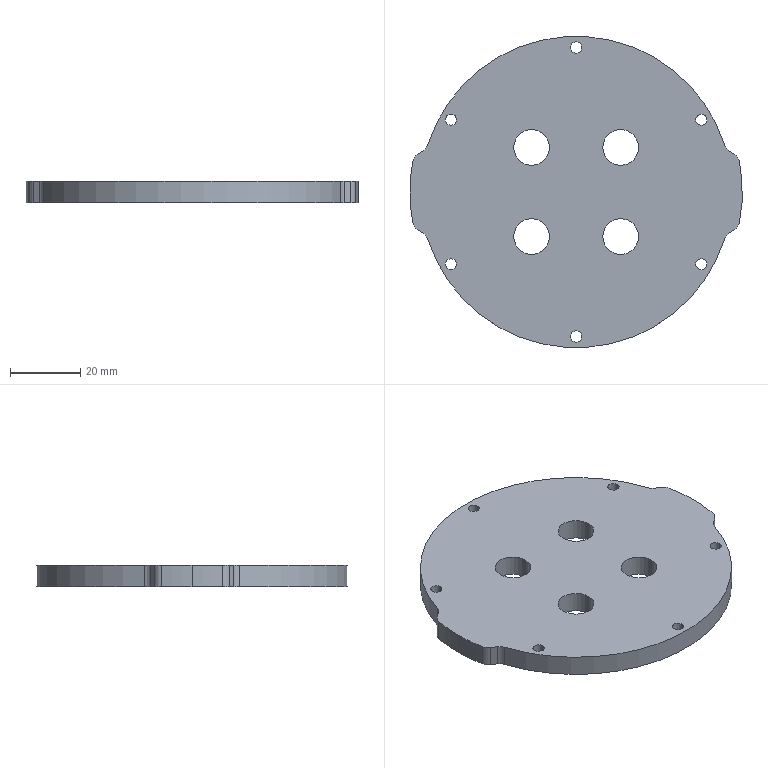Part | SolidWorks | features Extrusion 1 | 1 solid | 39 faces | box 94.9 x 88.9 x 6 mm | volume 35808 mm3 | cylinder 33 | plane 6 | commonest cylinder face diameters 3.2 x12 6 x8 10.2 x8 95 x3 88.9 x2
STEP:
#1=CARTESIAN_POINT('',(-1.55,41.275,6.));
#2=VERTEX_POINT('',#1);
#3=CARTESIAN_POINT('',(1.65,41.275,6.));
#4=VERTEX_POINT('',#3);
#5=CARTESIAN_POINT('',(0.05,41.275,6.));
#6=DIRECTION('',(0.,0.,1.));
#7=DIRECTION('',(1.,0.,0.));
#8=AXIS2_PLACEMENT_3D('',#5,#6,#7);
#9=CIRCLE('',#8,1.6);
#10=EDGE_CURVE('',#2,#4,#9,.T.);
#11=ORIENTED_EDGE('',*,*,#10,.T.);
#12=CARTESIAN_POINT('',(1.65,41.275,0.));
#13=VERTEX_POINT('',#12);
#14=CARTESIAN_POINT('',(1.65,41.275,6.));
#15=DIRECTION('',(0.,0.,-1.));
#16=VECTOR('',#15,1000.);
#17=LINE('',#14,#16);
#18=EDGE_CURVE('',#4,#13,#17,.T.);
#19=ORIENTED_EDGE('',*,*,#18,.T.);
#20=CARTESIAN_POINT('',(-1.55,41.275,0.));
#21=VERTEX_POINT('',#20);
#22=CARTESIAN_POINT('',(0.05,41.275,0.));
#23=DIRECTION('',(0.,0.,1.));
#24=DIRECTION('',(1.,0.,0.));
#25=AXIS2_PLACEMENT_3D('',#22,#23,#24);
#26=CIRCLE('',#25,1.6);
#27=EDGE_CURVE('',#21,#13,#26,.T.);
#28=ORIENTED_EDGE('',*,*,#27,.F.);
#29=CARTESIAN_POINT('',(-1.55,41.275,6.));
#30=DIRECTION('',(0.,0.,-1.));
#31=VECTOR('',#30,1000.);
#32=LINE('',#29,#31);
#33=EDGE_CURVE('',#2,#21,#32,.T.);
#34=ORIENTED_EDGE('',*,*,#33,.F.);
#35=EDGE_LOOP('',(#11,#19,#28,#34));
#36=FACE_OUTER_BOUND('',#35,.T.);
#37=CARTESIAN_POINT('',(0.05,41.275,6.));
#38=DIRECTION('',(0.,0.,-1.));
#39=DIRECTION('',(-1.,0.,0.));
#40=AXIS2_PLACEMENT_3D('',#37,#38,#39);
#41=CYLINDRICAL_SURFACE('',#40,1.6);
#42=ADVANCED_FACE('',(#36),#41,.F.);
#43=CARTESIAN_POINT('',(-1.55,-41.275,6.));
#44=VERTEX_POINT('',#43);
#45=CARTESIAN_POINT('',(1.65,-41.275,6.));
#46=VERTEX_POINT('',#45);
#47=CARTESIAN_POINT('',(0.05,-41.275,6.));
#48=DIRECTION('',(0.,0.,1.));
#49=DIRECTION('',(1.,0.,0.));
#50=AXIS2_PLACEMENT_3D('',#47,#48,#49);
#51=CIRCLE('',#50,1.6);
#52=EDGE_CURVE('',#44,#46,#51,.T.);
#53=ORIENTED_EDGE('',*,*,#52,.T.);
#54=CARTESIAN_POINT('',(1.65,-41.275,0.));
#55=VERTEX_POINT('',#54);
#56=CARTESIAN_POINT('',(1.65,-41.275,6.));
#57=DIRECTION('',(0.,0.,-1.));
#58=VECTOR('',#57,1000.);
#59=LINE('',#56,#58);
#60=EDGE_CURVE('',#46,#55,#59,.T.);
#61=ORIENTED_EDGE('',*,*,#60,.T.);
#62=CARTESIAN_POINT('',(-1.55,-41.275,0.));
#63=VERTEX_POINT('',#62);
#64=CARTESIAN_POINT('',(0.05,-41.275,0.));
#65=DIRECTION('',(0.,0.,1.));
#66=DIRECTION('',(1.,0.,0.));
#67=AXIS2_PLACEMENT_3D('',#64,#65,#66);
#68=CIRCLE('',#67,1.6);
#69=EDGE_CURVE('',#63,#55,#68,.T.);
#70=ORIENTED_EDGE('',*,*,#69,.F.);
#71=CARTESIAN_POINT('',(-1.55,-41.275,6.));
#72=DIRECTION('',(0.,0.,-1.));
#73=VECTOR('',#72,1000.);
#74=LINE('',#71,#73);
#75=EDGE_CURVE('',#44,#63,#74,.T.);
#76=ORIENTED_EDGE('',*,*,#75,.F.);
#77=EDGE_LOOP('',(#53,#61,#70,#76));
#78=FACE_OUTER_BOUND('',#77,.T.);
#79=CARTESIAN_POINT('',(0.05,-41.275,6.));
#80=DIRECTION('',(0.,0.,-1.));
#81=DIRECTION('',(-1.,0.,0.));
#82=AXIS2_PLACEMENT_3D('',#79,#80,#81);
#83=CYLINDRICAL_SURFACE('',#82,1.6);
#84=ADVANCED_FACE('',(#78),#83,.F.);
#85=CARTESIAN_POINT('',(-17.778,12.728,6.));
#86=VERTEX_POINT('',#85);
#87=CARTESIAN_POINT('',(-7.578,12.728,6.));
#88=VERTEX_POINT('',#87);
#89=CARTESIAN_POINT('',(-12.678,12.728,6.));
#90=DIRECTION('',(0.,0.,1.));
#91=DIRECTION('',(1.,0.,0.));
#92=AXIS2_PLACEMENT_3D('',#89,#90,#91);
#93=CIRCLE('',#92,5.1);
#94=EDGE_CURVE('',#86,#88,#93,.T.);
#95=ORIENTED_EDGE('',*,*,#94,.T.);
#96=CARTESIAN_POINT('',(-7.578,12.728,0.));
#97=VERTEX_POINT('',#96);
#98=CARTESIAN_POINT('',(-7.578,12.728,6.));
#99=DIRECTION('',(0.,0.,-1.));
#100=VECTOR('',#99,1000.);
#101=LINE('',#98,#100);
#102=EDGE_CURVE('',#88,#97,#101,.T.);
#103=ORIENTED_EDGE('',*,*,#102,.T.);
#104=CARTESIAN_POINT('',(-17.778,12.728,0.));
#105=VERTEX_POINT('',#104);
#106=CARTESIAN_POINT('',(-12.678,12.728,0.));
#107=DIRECTION('',(0.,0.,1.));
#108=DIRECTION('',(1.,0.,0.));
#109=AXIS2_PLACEMENT_3D('',#106,#107,#108);
#110=CIRCLE('',#109,5.1);
#111=EDGE_CURVE('',#105,#97,#110,.T.);
#112=ORIENTED_EDGE('',*,*,#111,.F.);
#113=CARTESIAN_POINT('',(-17.778,12.728,6.));
#114=DIRECTION('',(0.,0.,-1.));
#115=VECTOR('',#114,1000.);
#116=LINE('',#113,#115);
#117=EDGE_CURVE('',#86,#105,#116,.T.);
#118=ORIENTED_EDGE('',*,*,#117,.F.);
#119=EDGE_LOOP('',(#95,#103,#112,#118));
#120=FACE_OUTER_BOUND('',#119,.T.);
#121=CARTESIAN_POINT('',(-12.678,12.728,6.));
#122=DIRECTION('',(0.,0.,-1.));
#123=DIRECTION('',(-1.,0.,0.));
#124=AXIS2_PLACEMENT_3D('',#121,#122,#123);
#125=CYLINDRICAL_SURFACE('',#124,5.1);
#126=ADVANCED_FACE('',(#120),#125,.F.);
#127=CARTESIAN_POINT('',(-17.778,-12.728,6.));
#128=VERTEX_POINT('',#127);
#129=CARTESIAN_POINT('',(-7.578,-12.728,6.));
#130=VERTEX_POINT('',#129);
#131=CARTESIAN_POINT('',(-12.678,-12.728,6.));
#132=DIRECTION('',(0.,0.,1.));
#133=DIRECTION('',(1.,0.,0.));
#134=AXIS2_PLACEMENT_3D('',#131,#132,#133);
#135=CIRCLE('',#134,5.1);
#136=EDGE_CURVE('',#128,#130,#135,.T.);
#137=ORIENTED_EDGE('',*,*,#136,.T.);
#138=CARTESIAN_POINT('',(-7.578,-12.728,0.));
#139=VERTEX_POINT('',#138);
#140=CARTESIAN_POINT('',(-7.578,-12.728,6.));
#141=DIRECTION('',(0.,0.,-1.));
#142=VECTOR('',#141,1000.);
#143=LINE('',#140,#142);
#144=EDGE_CURVE('',#130,#139,#143,.T.);
#145=ORIENTED_EDGE('',*,*,#144,.T.);
#146=CARTESIAN_POINT('',(-17.778,-12.728,0.));
#147=VERTEX_POINT('',#146);
#148=CARTESIAN_POINT('',(-12.678,-12.728,0.));
#149=DIRECTION('',(0.,0.,1.));
#150=DIRECTION('',(1.,0.,0.));
#151=AXIS2_PLACEMENT_3D('',#148,#149,#150);
#152=CIRCLE('',#151,5.1);
#153=EDGE_CURVE('',#147,#139,#152,.T.);
#154=ORIENTED_EDGE('',*,*,#153,.F.);
#155=CARTESIAN_POINT('',(-17.778,-12.728,6.));
#156=DIRECTION('',(0.,0.,-1.));
#157=VECTOR('',#156,1000.);
#158=LINE('',#155,#157);
#159=EDGE_CURVE('',#128,#147,#158,.T.);
#160=ORIENTED_EDGE('',*,*,#159,.F.);
#161=EDGE_LOOP('',(#137,#145,#154,#160));
#162=FACE_OUTER_BOUND('',#161,.T.);
#163=CARTESIAN_POINT('',(-12.678,-12.728,6.));
#164=DIRECTION('',(0.,0.,-1.));
#165=DIRECTION('',(-1.,0.,0.));
#166=AXIS2_PLACEMENT_3D('',#163,#164,#165);
#167=CYLINDRICAL_SURFACE('',#166,5.1);
#168=ADVANCED_FACE('',(#162),#167,.F.);
#169=CARTESIAN_POINT('',(7.678,-12.728,6.));
#170=VERTEX_POINT('',#169);
#171=CARTESIAN_POINT('',(17.878,-12.728,6.));
#172=VERTEX_POINT('',#171);
#173=CARTESIAN_POINT('',(12.778,-12.728,6.));
#174=DIRECTION('',(0.,0.,1.));
#175=DIRECTION('',(1.,0.,0.));
#176=AXIS2_PLACEMENT_3D('',#173,#174,#175);
#177=CIRCLE('',#176,5.1);
#178=EDGE_CURVE('',#170,#172,#177,.T.);
#179=ORIENTED_EDGE('',*,*,#178,.T.);
#180=CARTESIAN_POINT('',(17.878,-12.728,0.));
#181=VERTEX_POINT('',#180);
#182=CARTESIAN_POINT('',(17.878,-12.728,6.));
#183=DIRECTION('',(0.,0.,-1.));
#184=VECTOR('',#183,1000.);
#185=LINE('',#182,#184);
#186=EDGE_CURVE('',#172,#181,#185,.T.);
#187=ORIENTED_EDGE('',*,*,#186,.T.);
#188=CARTESIAN_POINT('',(7.678,-12.728,0.));
#189=VERTEX_POINT('',#188);
#190=CARTESIAN_POINT('',(12.778,-12.728,0.));
#191=DIRECTION('',(0.,0.,1.));
#192=DIRECTION('',(1.,0.,0.));
#193=AXIS2_PLACEMENT_3D('',#190,#191,#192);
#194=CIRCLE('',#193,5.1);
#195=EDGE_CURVE('',#189,#181,#194,.T.);
#196=ORIENTED_EDGE('',*,*,#195,.F.);
#197=CARTESIAN_POINT('',(7.678,-12.728,6.));
#198=DIRECTION('',(0.,0.,-1.));
#199=VECTOR('',#198,1000.);
#200=LINE('',#197,#199);
#201=EDGE_CURVE('',#170,#189,#200,.T.);
#202=ORIENTED_EDGE('',*,*,#201,.F.);
#203=EDGE_LOOP('',(#179,#187,#196,#202));
#204=FACE_OUTER_BOUND('',#203,.T.);
#205=CARTESIAN_POINT('',(12.778,-12.728,6.));
#206=DIRECTION('',(0.,0.,-1.));
#207=DIRECTION('',(-1.,0.,0.));
#208=AXIS2_PLACEMENT_3D('',#205,#206,#207);
#209=CYLINDRICAL_SURFACE('',#208,5.1);
#210=ADVANCED_FACE('',(#204),#209,.F.);
#211=CARTESIAN_POINT('',(7.678,12.728,6.));
#212=VERTEX_POINT('',#211);
#213=CARTESIAN_POINT('',(17.878,12.728,6.));
#214=VERTEX_POINT('',#213);
#215=CARTESIAN_POINT('',(12.778,12.728,6.));
#216=DIRECTION('',(0.,0.,1.));
#217=DIRECTION('',(1.,0.,0.));
#218=AXIS2_PLACEMENT_3D('',#215,#216,#217);
#219=CIRCLE('',#218,5.1);
#220=EDGE_CURVE('',#212,#214,#219,.T.);
#221=ORIENTED_EDGE('',*,*,#220,.T.);
#222=CARTESIAN_POINT('',(17.878,12.728,0.));
#223=VERTEX_POINT('',#222);
#224=CARTESIAN_POINT('',(17.878,12.728,6.));
#225=DIRECTION('',(0.,0.,-1.));
#226=VECTOR('',#225,1000.);
#227=LINE('',#224,#226);
#228=EDGE_CURVE('',#214,#223,#227,.T.);
#229=ORIENTED_EDGE('',*,*,#228,.T.);
#230=CARTESIAN_POINT('',(7.678,12.728,0.));
#231=VERTEX_POINT('',#230);
#232=CARTESIAN_POINT('',(12.778,12.728,0.));
#233=DIRECTION('',(0.,0.,1.));
#234=DIRECTION('',(1.,0.,0.));
#235=AXIS2_PLACEMENT_3D('',#232,#233,#234);
#236=CIRCLE('',#235,5.1);
#237=EDGE_CURVE('',#231,#223,#236,.T.);
#238=ORIENTED_EDGE('',*,*,#237,.F.);
#239=CARTESIAN_POINT('',(7.678,12.728,6.));
#240=DIRECTION('',(0.,0.,-1.));
#241=VECTOR('',#240,1000.);
#242=LINE('',#239,#241);
#243=EDGE_CURVE('',#212,#231,#242,.T.);
#244=ORIENTED_EDGE('',*,*,#243,.F.);
#245=EDGE_LOOP('',(#221,#229,#238,#244));
#246=FACE_OUTER_BOUND('',#245,.T.);
#247=CARTESIAN_POINT('',(12.778,12.728,6.));
#248=DIRECTION('',(0.,0.,-1.));
#249=DIRECTION('',(-1.,0.,0.));
#250=AXIS2_PLACEMENT_3D('',#247,#248,#249);
#251=CYLINDRICAL_SURFACE('',#250,5.1);
#252=ADVANCED_FACE('',(#246),#251,.F.);
#253=CARTESIAN_POINT('',(34.195,20.637,6.));
#254=VERTEX_POINT('',#253);
#255=CARTESIAN_POINT('',(37.395,20.637,6.));
#256=VERTEX_POINT('',#255);
#257=CARTESIAN_POINT('',(35.795,20.637,6.));
#258=DIRECTION('',(0.,0.,1.));
#259=DIRECTION('',(1.,0.,0.));
#260=AXIS2_PLACEMENT_3D('',#257,#258,#259);
#261=CIRCLE('',#260,1.6);
#262=EDGE_CURVE('',#254,#256,#261,.T.);
#263=ORIENTED_EDGE('',*,*,#262,.T.);
#264=CARTESIAN_POINT('',(37.395,20.637,0.));
#265=VERTEX_POINT('',#264);
#266=CARTESIAN_POINT('',(37.395,20.637,6.));
#267=DIRECTION('',(0.,0.,-1.));
#268=VECTOR('',#267,1000.);
#269=LINE('',#266,#268);
#270=EDGE_CURVE('',#256,#265,#269,.T.);
#271=ORIENTED_EDGE('',*,*,#270,.T.);
#272=CARTESIAN_POINT('',(34.195,20.637,0.));
#273=VERTEX_POINT('',#272);
#274=CARTESIAN_POINT('',(35.795,20.637,0.));
#275=DIRECTION('',(0.,0.,1.));
#276=DIRECTION('',(1.,0.,0.));
#277=AXIS2_PLACEMENT_3D('',#274,#275,#276);
#278=CIRCLE('',#277,1.6);
#279=EDGE_CURVE('',#273,#265,#278,.T.);
#280=ORIENTED_EDGE('',*,*,#279,.F.);
#281=CARTESIAN_POINT('',(34.195,20.637,6.));
#282=DIRECTION('',(0.,0.,-1.));
#283=VECTOR('',#282,1000.);
#284=LINE('',#281,#283);
#285=EDGE_CURVE('',#254,#273,#284,.T.);
#286=ORIENTED_EDGE('',*,*,#285,.F.);
#287=EDGE_LOOP('',(#263,#271,#280,#286));
#288=FACE_OUTER_BOUND('',#287,.T.);
#289=CARTESIAN_POINT('',(35.795,20.637,6.));
#290=DIRECTION('',(0.,0.,-1.));
#291=DIRECTION('',(-1.,0.,0.));
#292=AXIS2_PLACEMENT_3D('',#289,#290,#291);
#293=CYLINDRICAL_SURFACE('',#292,1.6);
#294=ADVANCED_FACE('',(#288),#293,.F.);
#295=CARTESIAN_POINT('',(34.195,-20.638,6.));
#296=VERTEX_POINT('',#295);
#297=CARTESIAN_POINT('',(37.395,-20.638,6.));
#298=VERTEX_POINT('',#297);
#299=CARTESIAN_POINT('',(35.795,-20.638,6.));
#300=DIRECTION('',(0.,0.,1.));
#301=DIRECTION('',(1.,0.,0.));
#302=AXIS2_PLACEMENT_3D('',#299,#300,#301);
#303=CIRCLE('',#302,1.6);
#304=EDGE_CURVE('',#296,#298,#303,.T.);
#305=ORIENTED_EDGE('',*,*,#304,.T.);
#306=CARTESIAN_POINT('',(37.395,-20.638,0.));
#307=VERTEX_POINT('',#306);
#308=CARTESIAN_POINT('',(37.395,-20.638,6.));
#309=DIRECTION('',(0.,0.,-1.));
#310=VECTOR('',#309,1000.);
#311=LINE('',#308,#310);
#312=EDGE_CURVE('',#298,#307,#311,.T.);
#313=ORIENTED_EDGE('',*,*,#312,.T.);
#314=CARTESIAN_POINT('',(34.195,-20.638,0.));
#315=VERTEX_POINT('',#314);
#316=CARTESIAN_POINT('',(35.795,-20.638,0.));
#317=DIRECTION('',(0.,0.,1.));
#318=DIRECTION('',(1.,0.,0.));
#319=AXIS2_PLACEMENT_3D('',#316,#317,#318);
#320=CIRCLE('',#319,1.6);
#321=EDGE_CURVE('',#315,#307,#320,.T.);
#322=ORIENTED_EDGE('',*,*,#321,.F.);
#323=CARTESIAN_POINT('',(34.195,-20.638,6.));
#324=DIRECTION('',(0.,0.,-1.));
#325=VECTOR('',#324,1000.);
#326=LINE('',#323,#325);
#327=EDGE_CURVE('',#296,#315,#326,.T.);
#328=ORIENTED_EDGE('',*,*,#327,.F.);
#329=EDGE_LOOP('',(#305,#313,#322,#328));
#330=FACE_OUTER_BOUND('',#329,.T.);
#331=CARTESIAN_POINT('',(35.795,-20.638,6.));
#332=DIRECTION('',(0.,0.,-1.));
#333=DIRECTION('',(-1.,0.,0.));
#334=AXIS2_PLACEMENT_3D('',#331,#332,#333);
#335=CYLINDRICAL_SURFACE('',#334,1.6);
#336=ADVANCED_FACE('',(#330),#335,.F.);
#337=CARTESIAN_POINT('',(-37.295,-20.637,6.));
#338=VERTEX_POINT('',#337);
#339=CARTESIAN_POINT('',(-34.095,-20.637,6.));
#340=VERTEX_POINT('',#339);
#341=CARTESIAN_POINT('',(-35.695,-20.637,6.));
#342=DIRECTION('',(0.,0.,1.));
#343=DIRECTION('',(1.,0.,0.));
#344=AXIS2_PLACEMENT_3D('',#341,#342,#343);
#345=CIRCLE('',#344,1.6);
#346=EDGE_CURVE('',#338,#340,#345,.T.);
#347=ORIENTED_EDGE('',*,*,#346,.T.);
#348=CARTESIAN_POINT('',(-34.095,-20.637,0.));
#349=VERTEX_POINT('',#348);
#350=CARTESIAN_POINT('',(-34.095,-20.637,6.));
#351=DIRECTION('',(0.,0.,-1.));
#352=VECTOR('',#351,1000.);
#353=LINE('',#350,#352);
#354=EDGE_CURVE('',#340,#349,#353,.T.);
#355=ORIENTED_EDGE('',*,*,#354,.T.);
#356=CARTESIAN_POINT('',(-37.295,-20.637,0.));
#357=VERTEX_POINT('',#356);
#358=CARTESIAN_POINT('',(-35.695,-20.637,0.));
#359=DIRECTION('',(0.,0.,1.));
#360=DIRECTION('',(1.,0.,0.));
#361=AXIS2_PLACEMENT_3D('',#358,#359,#360);
#362=CIRCLE('',#361,1.6);
#363=EDGE_CURVE('',#357,#349,#362,.T.);
#364=ORIENTED_EDGE('',*,*,#363,.F.);
#365=CARTESIAN_POINT('',(-37.295,-20.637,6.));
#366=DIRECTION('',(0.,0.,-1.));
#367=VECTOR('',#366,1000.);
#368=LINE('',#365,#367);
#369=EDGE_CURVE('',#338,#357,#368,.T.);
#370=ORIENTED_EDGE('',*,*,#369,.F.);
#371=EDGE_LOOP('',(#347,#355,#364,#370));
#372=FACE_OUTER_BOUND('',#371,.T.);
#373=CARTESIAN_POINT('',(-35.695,-20.637,6.));
#374=DIRECTION('',(0.,0.,-1.));
#375=DIRECTION('',(-1.,0.,0.));
#376=AXIS2_PLACEMENT_3D('',#373,#374,#375);
#377=CYLINDRICAL_SURFACE('',#376,1.6);
#378=ADVANCED_FACE('',(#372),#377,.F.);
#379=CARTESIAN_POINT('',(-37.295,20.638,6.));
#380=VERTEX_POINT('',#379);
#381=CARTESIAN_POINT('',(-34.095,20.638,6.));
#382=VERTEX_POINT('',#381);
#383=CARTESIAN_POINT('',(-35.695,20.638,6.));
#384=DIRECTION('',(0.,0.,1.));
#385=DIRECTION('',(1.,0.,0.));
#386=AXIS2_PLACEMENT_3D('',#383,#384,#385);
#387=CIRCLE('',#386,1.6);
#388=EDGE_CURVE('',#380,#382,#387,.T.);
#389=ORIENTED_EDGE('',*,*,#388,.T.);
#390=CARTESIAN_POINT('',(-34.095,20.638,0.));
#391=VERTEX_POINT('',#390);
#392=CARTESIAN_POINT('',(-34.095,20.638,6.));
#393=DIRECTION('',(0.,0.,-1.));
#394=VECTOR('',#393,1000.);
#395=LINE('',#392,#394);
#396=EDGE_CURVE('',#382,#391,#395,.T.);
#397=ORIENTED_EDGE('',*,*,#396,.T.);
#398=CARTESIAN_POINT('',(-37.295,20.638,0.));
#399=VERTEX_POINT('',#398);
#400=CARTESIAN_POINT('',(-35.695,20.638,0.));
#401=DIRECTION('',(0.,0.,1.));
#402=DIRECTION('',(1.,0.,0.));
#403=AXIS2_PLACEMENT_3D('',#400,#401,#402);
#404=CIRCLE('',#403,1.6);
#405=EDGE_CURVE('',#399,#391,#404,.T.);
#406=ORIENTED_EDGE('',*,*,#405,.F.);
#407=CARTESIAN_POINT('',(-37.295,20.638,6.));
#408=DIRECTION('',(0.,0.,-1.));
#409=VECTOR('',#408,1000.);
#410=LINE('',#407,#409);
#411=EDGE_CURVE('',#380,#399,#410,.T.);
#412=ORIENTED_EDGE('',*,*,#411,.F.);
#413=EDGE_LOOP('',(#389,#397,#406,#412));
#414=FACE_OUTER_BOUND('',#413,.T.);
#415=CARTESIAN_POINT('',(-35.695,20.638,6.));
#416=DIRECTION('',(0.,0.,-1.));
#417=DIRECTION('',(-1.,0.,0.));
#418=AXIS2_PLACEMENT_3D('',#415,#416,#417);
#419=CYLINDRICAL_SURFACE('',#418,1.6);
#420=ADVANCED_FACE('',(#414),#419,.F.);
#421=CARTESIAN_POINT('',(-47.4,0.,6.));
#422=VERTEX_POINT('',#421);
#423=CARTESIAN_POINT('',(-46.587,-8.749,6.));
#424=VERTEX_POINT('',#423);
#425=CARTESIAN_POINT('',(0.1,0.,6.));
#426=DIRECTION('',(0.,0.,1.));
#427=DIRECTION('',(1.,0.,0.));
#428=AXIS2_PLACEMENT_3D('',#425,#426,#427);
#429=CIRCLE('',#428,47.5);
#430=EDGE_CURVE('',#422,#424,#429,.T.);
#431=ORIENTED_EDGE('',*,*,#430,.F.);
#432=CARTESIAN_POINT('',(-47.4,0.,0.));
#433=VERTEX_POINT('',#432);
#434=CARTESIAN_POINT('',(-47.4,0.,6.));
#435=DIRECTION('',(0.,0.,-1.));
#436=VECTOR('',#435,1000.);
#437=LINE('',#434,#436);
#438=EDGE_CURVE('',#422,#433,#437,.T.);
#439=ORIENTED_EDGE('',*,*,#438,.T.);
#440=CARTESIAN_POINT('',(-46.587,-8.749,0.));
#441=VERTEX_POINT('',#440);
#442=CARTESIAN_POINT('',(0.1,0.,0.));
#443=DIRECTION('',(0.,0.,1.));
#444=DIRECTION('',(1.,0.,0.));
#445=AXIS2_PLACEMENT_3D('',#442,#443,#444);
#446=CIRCLE('',#445,47.5);
#447=EDGE_CURVE('',#433,#441,#446,.T.);
#448=ORIENTED_EDGE('',*,*,#447,.T.);
#449=CARTESIAN_POINT('',(-46.587,-8.749,6.));
#450=DIRECTION('',(0.,0.,-1.));
#451=VECTOR('',#450,1000.);
#452=LINE('',#449,#451);
#453=EDGE_CURVE('',#424,#441,#452,.T.);
#454=ORIENTED_EDGE('',*,*,#453,.F.);
#455=EDGE_LOOP('',(#431,#439,#448,#454));
#456=FACE_OUTER_BOUND('',#455,.T.);
#457=CARTESIAN_POINT('',(0.1,0.,6.));
#458=DIRECTION('',(0.,0.,-1.));
#459=DIRECTION('',(-1.,0.,0.));
#460=AXIS2_PLACEMENT_3D('',#457,#458,#459);
#461=CYLINDRICAL_SURFACE('',#460,47.5);
#462=ADVANCED_FACE('',(#456),#461,.T.);
#463=ORIENTED_EDGE('',*,*,#52,.F.);
#464=CARTESIAN_POINT('',(0.05,-41.275,6.));
#465=DIRECTION('',(0.,0.,1.));
#466=DIRECTION('',(1.,0.,0.));
#467=AXIS2_PLACEMENT_3D('',#464,#465,#466);
#468=CIRCLE('',#467,1.6);
#469=EDGE_CURVE('',#46,#44,#468,.T.);
#470=ORIENTED_EDGE('',*,*,#469,.F.);
#471=EDGE_LOOP('',(#463,#470));
#472=FACE_BOUND('',#471,.T.);
#473=ORIENTED_EDGE('',*,*,#136,.F.);
#474=CARTESIAN_POINT('',(-12.678,-12.728,6.));
#475=DIRECTION('',(0.,0.,1.));
#476=DIRECTION('',(1.,0.,0.));
#477=AXIS2_PLACEMENT_3D('',#474,#475,#476);
#478=CIRCLE('',#477,5.1);
#479=EDGE_CURVE('',#130,#128,#478,.T.);
#480=ORIENTED_EDGE('',*,*,#479,.F.);
#481=EDGE_LOOP('',(#473,#480));
#482=FACE_BOUND('',#481,.T.);
#483=ORIENTED_EDGE('',*,*,#220,.F.);
#484=CARTESIAN_POINT('',(12.778,12.728,6.));
#485=DIRECTION('',(0.,0.,1.));
#486=DIRECTION('',(1.,0.,0.));
#487=AXIS2_PLACEMENT_3D('',#484,#485,#486);
#488=CIRCLE('',#487,5.1);
#489=EDGE_CURVE('',#214,#212,#488,.T.);
#490=ORIENTED_EDGE('',*,*,#489,.F.);
#491=EDGE_LOOP('',(#483,#490));
#492=FACE_BOUND('',#491,.T.);
#493=ORIENTED_EDGE('',*,*,#304,.F.);
#494=CARTESIAN_POINT('',(35.795,-20.638,6.));
#495=DIRECTION('',(0.,0.,1.));
#496=DIRECTION('',(1.,0.,0.));
#497=AXIS2_PLACEMENT_3D('',#494,#495,#496);
#498=CIRCLE('',#497,1.6);
#499=EDGE_CURVE('',#298,#296,#498,.T.);
#500=ORIENTED_EDGE('',*,*,#499,.F.);
#501=EDGE_LOOP('',(#493,#500));
#502=FACE_BOUND('',#501,.T.);
#503=ORIENTED_EDGE('',*,*,#388,.F.);
#504=CARTESIAN_POINT('',(-35.695,20.638,6.));
#505=DIRECTION('',(0.,0.,1.));
#506=DIRECTION('',(1.,0.,0.));
#507=AXIS2_PLACEMENT_3D('',#504,#505,#506);
#508=CIRCLE('',#507,1.6);
#509=EDGE_CURVE('',#382,#380,#508,.T.);
#510=ORIENTED_EDGE('',*,*,#509,.F.);
#511=EDGE_LOOP('',(#503,#510));
#512=FACE_BOUND('',#511,.T.);
#513=CARTESIAN_POINT('',(-45.309,10.688,6.));
#514=VERTEX_POINT('',#513);
#515=CARTESIAN_POINT('',(-46.587,8.749,6.));
#516=VERTEX_POINT('',#515);
#517=CARTESIAN_POINT('',(-43.639,8.196,6.));
#518=DIRECTION('',(0.,0.,1.));
#519=DIRECTION('',(1.,0.,0.));
#520=AXIS2_PLACEMENT_3D('',#517,#518,#519);
#521=CIRCLE('',#520,3.);
#522=EDGE_CURVE('',#514,#516,#521,.T.);
#523=ORIENTED_EDGE('',*,*,#522,.T.);
#524=CARTESIAN_POINT('',(0.1,0.,6.));
#525=DIRECTION('',(0.,0.,1.));
#526=DIRECTION('',(1.,0.,0.));
#527=AXIS2_PLACEMENT_3D('',#524,#525,#526);
#528=CIRCLE('',#527,47.5);
#529=EDGE_CURVE('',#516,#422,#528,.T.);
#530=ORIENTED_EDGE('',*,*,#529,.T.);
#531=ORIENTED_EDGE('',*,*,#430,.T.);
#532=CARTESIAN_POINT('',(-45.309,-10.688,6.));
#533=VERTEX_POINT('',#532);
#534=CARTESIAN_POINT('',(-43.639,-8.196,6.));
#535=DIRECTION('',(0.,0.,1.));
#536=DIRECTION('',(1.,0.,0.));
#537=AXIS2_PLACEMENT_3D('',#534,#535,#536);
#538=CIRCLE('',#537,3.);
#539=EDGE_CURVE('',#424,#533,#538,.T.);
#540=ORIENTED_EDGE('',*,*,#539,.T.);
#541=CARTESIAN_POINT('',(-43.492,-11.906,6.));
#542=VERTEX_POINT('',#541);
#543=CARTESIAN_POINT('',(-45.309,-10.688,6.));
#544=DIRECTION('',(0.8306,-0.5568,0.));
#545=VECTOR('',#544,1000.);
#546=LINE('',#543,#545);
#547=EDGE_CURVE('',#533,#542,#546,.T.);
#548=ORIENTED_EDGE('',*,*,#547,.T.);
#549=CARTESIAN_POINT('',(-42.304,-13.487,6.));
#550=VERTEX_POINT('',#549);
#551=CARTESIAN_POINT('',(-45.163,-14.398,6.));
#552=DIRECTION('',(0.,0.,-1.));
#553=DIRECTION('',(1.,0.,0.));
#554=AXIS2_PLACEMENT_3D('',#551,#552,#553);
#555=CIRCLE('',#554,3.);
#556=EDGE_CURVE('',#542,#550,#555,.T.);
#557=ORIENTED_EDGE('',*,*,#556,.T.);
#558=CARTESIAN_POINT('',(42.404,-13.487,6.));
#559=VERTEX_POINT('',#558);
#560=CARTESIAN_POINT('',(0.05,0.,6.));
#561=DIRECTION('',(0.,0.,1.));
#562=DIRECTION('',(1.,0.,0.));
#563=AXIS2_PLACEMENT_3D('',#560,#561,#562);
#564=CIRCLE('',#563,44.45);
#565=EDGE_CURVE('',#550,#559,#564,.T.);
#566=ORIENTED_EDGE('',*,*,#565,.T.);
#567=CARTESIAN_POINT('',(43.592,-11.906,6.));
#568=VERTEX_POINT('',#567);
#569=CARTESIAN_POINT('',(45.263,-14.398,6.));
#570=DIRECTION('',(0.,0.,-1.));
#571=DIRECTION('',(1.,0.,0.));
#572=AXIS2_PLACEMENT_3D('',#569,#570,#571);
#573=CIRCLE('',#572,3.);
#574=EDGE_CURVE('',#559,#568,#573,.T.);
#575=ORIENTED_EDGE('',*,*,#574,.T.);
#576=CARTESIAN_POINT('',(45.409,-10.688,6.));
#577=VERTEX_POINT('',#576);
#578=CARTESIAN_POINT('',(43.592,-11.906,6.));
#579=DIRECTION('',(0.8306,0.5568,0.));
#580=VECTOR('',#579,1000.);
#581=LINE('',#578,#580);
#582=EDGE_CURVE('',#568,#577,#581,.T.);
#583=ORIENTED_EDGE('',*,*,#582,.T.);
#584=CARTESIAN_POINT('',(46.687,-8.749,6.));
#585=VERTEX_POINT('',#584);
#586=CARTESIAN_POINT('',(43.739,-8.196,6.));
#587=DIRECTION('',(0.,0.,1.));
#588=DIRECTION('',(1.,0.,0.));
#589=AXIS2_PLACEMENT_3D('',#586,#587,#588);
#590=CIRCLE('',#589,3.);
#591=EDGE_CURVE('',#577,#585,#590,.T.);
#592=ORIENTED_EDGE('',*,*,#591,.T.);
#593=CARTESIAN_POINT('',(46.687,8.749,6.));
#594=VERTEX_POINT('',#593);
#595=CARTESIAN_POINT('',(0.,0.,6.));
#596=DIRECTION('',(0.,0.,1.));
#597=DIRECTION('',(1.,0.,0.));
#598=AXIS2_PLACEMENT_3D('',#595,#596,#597);
#599=CIRCLE('',#598,47.5);
#600=EDGE_CURVE('',#585,#594,#599,.T.);
#601=ORIENTED_EDGE('',*,*,#600,.T.);
#602=CARTESIAN_POINT('',(45.409,10.688,6.));
#603=VERTEX_POINT('',#602);
#604=CARTESIAN_POINT('',(43.739,8.196,6.));
#605=DIRECTION('',(0.,0.,1.));
#606=DIRECTION('',(1.,0.,0.));
#607=AXIS2_PLACEMENT_3D('',#604,#605,#606);
#608=CIRCLE('',#607,3.);
#609=EDGE_CURVE('',#594,#603,#608,.T.);
#610=ORIENTED_EDGE('',*,*,#609,.T.);
#611=CARTESIAN_POINT('',(43.592,11.906,6.));
#612=VERTEX_POINT('',#611);
#613=CARTESIAN_POINT('',(45.409,10.688,6.));
#614=DIRECTION('',(-0.8306,0.5568,0.));
#615=VECTOR('',#614,1000.);
#616=LINE('',#613,#615);
#617=EDGE_CURVE('',#603,#612,#616,.T.);
#618=ORIENTED_EDGE('',*,*,#617,.T.);
#619=CARTESIAN_POINT('',(42.404,13.487,6.));
#620=VERTEX_POINT('',#619);
#621=CARTESIAN_POINT('',(45.263,14.398,6.));
#622=DIRECTION('',(0.,0.,-1.));
#623=DIRECTION('',(1.,0.,0.));
#624=AXIS2_PLACEMENT_3D('',#621,#622,#623);
#625=CIRCLE('',#624,3.);
#626=EDGE_CURVE('',#612,#620,#625,.T.);
#627=ORIENTED_EDGE('',*,*,#626,.T.);
#628=CARTESIAN_POINT('',(-42.304,13.487,6.));
#629=VERTEX_POINT('',#628);
#630=CARTESIAN_POINT('',(0.05,0.,6.));
#631=DIRECTION('',(0.,0.,1.));
#632=DIRECTION('',(1.,0.,0.));
#633=AXIS2_PLACEMENT_3D('',#630,#631,#632);
#634=CIRCLE('',#633,44.45);
#635=EDGE_CURVE('',#620,#629,#634,.T.);
#636=ORIENTED_EDGE('',*,*,#635,.T.);
#637=CARTESIAN_POINT('',(-43.492,11.906,6.));
#638=VERTEX_POINT('',#637);
#639=CARTESIAN_POINT('',(-45.163,14.398,6.));
#640=DIRECTION('',(0.,0.,-1.));
#641=DIRECTION('',(1.,0.,0.));
#642=AXIS2_PLACEMENT_3D('',#639,#640,#641);
#643=CIRCLE('',#642,3.);
#644=EDGE_CURVE('',#629,#638,#643,.T.);
#645=ORIENTED_EDGE('',*,*,#644,.T.);
#646=CARTESIAN_POINT('',(-43.492,11.906,6.));
#647=DIRECTION('',(-0.8306,-0.5568,0.));
#648=VECTOR('',#647,1000.);
#649=LINE('',#646,#648);
#650=EDGE_CURVE('',#638,#514,#649,.T.);
#651=ORIENTED_EDGE('',*,*,#650,.T.);
#652=EDGE_LOOP('',(#523,#530,#531,#540,#548,#557,#566,#575,#583,#592,#601,#610,#618,#627,#636,#645,#651));
#653=FACE_OUTER_BOUND('',#652,.T.);
#654=ORIENTED_EDGE('',*,*,#346,.F.);
#655=CARTESIAN_POINT('',(-35.695,-20.637,6.));
#656=DIRECTION('',(0.,0.,1.));
#657=DIRECTION('',(1.,0.,0.));
#658=AXIS2_PLACEMENT_3D('',#655,#656,#657);
#659=CIRCLE('',#658,1.6);
#660=EDGE_CURVE('',#340,#338,#659,.T.);
#661=ORIENTED_EDGE('',*,*,#660,.F.);
#662=EDGE_LOOP('',(#654,#661));
#663=FACE_BOUND('',#662,.T.);
#664=ORIENTED_EDGE('',*,*,#262,.F.);
#665=CARTESIAN_POINT('',(35.795,20.637,6.));
#666=DIRECTION('',(0.,0.,1.));
#667=DIRECTION('',(1.,0.,0.));
#668=AXIS2_PLACEMENT_3D('',#665,#666,#667);
#669=CIRCLE('',#668,1.6);
#670=EDGE_CURVE('',#256,#254,#669,.T.);
#671=ORIENTED_EDGE('',*,*,#670,.F.);
#672=EDGE_LOOP('',(#664,#671));
#673=FACE_BOUND('',#672,.T.);
#674=ORIENTED_EDGE('',*,*,#178,.F.);
#675=CARTESIAN_POINT('',(12.778,-12.728,6.));
#676=DIRECTION('',(0.,0.,1.));
#677=DIRECTION('',(1.,0.,0.));
#678=AXIS2_PLACEMENT_3D('',#675,#676,#677);
#679=CIRCLE('',#678,5.1);
#680=EDGE_CURVE('',#172,#170,#679,.T.);
#681=ORIENTED_EDGE('',*,*,#680,.F.);
#682=EDGE_LOOP('',(#674,#681));
#683=FACE_BOUND('',#682,.T.);
#684=ORIENTED_EDGE('',*,*,#94,.F.);
#685=CARTESIAN_POINT('',(-12.678,12.728,6.));
#686=DIRECTION('',(0.,0.,1.));
#687=DIRECTION('',(1.,0.,0.));
#688=AXIS2_PLACEMENT_3D('',#685,#686,#687);
#689=CIRCLE('',#688,5.1);
#690=EDGE_CURVE('',#88,#86,#689,.T.);
#691=ORIENTED_EDGE('',*,*,#690,.F.);
#692=EDGE_LOOP('',(#684,#691));
#693=FACE_BOUND('',#692,.T.);
#694=ORIENTED_EDGE('',*,*,#10,.F.);
#695=CARTESIAN_POINT('',(0.05,41.275,6.));
#696=DIRECTION('',(0.,0.,1.));
#697=DIRECTION('',(1.,0.,0.));
#698=AXIS2_PLACEMENT_3D('',#695,#696,#697);
#699=CIRCLE('',#698,1.6);
#700=EDGE_CURVE('',#4,#2,#699,.T.);
#701=ORIENTED_EDGE('',*,*,#700,.F.);
#702=EDGE_LOOP('',(#694,#701));
#703=FACE_BOUND('',#702,.T.);
#704=CARTESIAN_POINT('',(-43.639,8.196,6.));
#705=DIRECTION('',(0.,0.,1.));
#706=DIRECTION('',(1.,0.,0.));
#707=AXIS2_PLACEMENT_3D('',#704,#705,#706);
#708=PLANE('',#707);
#709=ADVANCED_FACE('',(#472,#482,#492,#502,#512,#653,#663,#673,#683,#693,#703),#708,.T.);
#710=CARTESIAN_POINT('',(-45.309,10.688,0.));
#711=VERTEX_POINT('',#710);
#712=CARTESIAN_POINT('',(-46.587,8.749,0.));
#713=VERTEX_POINT('',#712);
#714=CARTESIAN_POINT('',(-43.639,8.196,0.));
#715=DIRECTION('',(0.,0.,1.));
#716=DIRECTION('',(1.,0.,0.));
#717=AXIS2_PLACEMENT_3D('',#714,#715,#716);
#718=CIRCLE('',#717,3.);
#719=EDGE_CURVE('',#711,#713,#718,.T.);
#720=ORIENTED_EDGE('',*,*,#719,.F.);
#721=CARTESIAN_POINT('',(-43.492,11.906,0.));
#722=VERTEX_POINT('',#721);
#723=CARTESIAN_POINT('',(-43.492,11.906,0.));
#724=DIRECTION('',(-0.8306,-0.5568,0.));
#725=VECTOR('',#724,1000.);
#726=LINE('',#723,#725);
#727=EDGE_CURVE('',#722,#711,#726,.T.);
#728=ORIENTED_EDGE('',*,*,#727,.F.);
#729=CARTESIAN_POINT('',(-42.304,13.487,0.));
#730=VERTEX_POINT('',#729);
#731=CARTESIAN_POINT('',(-45.163,14.398,0.));
#732=DIRECTION('',(0.,0.,-1.));
#733=DIRECTION('',(1.,0.,0.));
#734=AXIS2_PLACEMENT_3D('',#731,#732,#733);
#735=CIRCLE('',#734,3.);
#736=EDGE_CURVE('',#730,#722,#735,.T.);
#737=ORIENTED_EDGE('',*,*,#736,.F.);
#738=CARTESIAN_POINT('',(42.404,13.487,0.));
#739=VERTEX_POINT('',#738);
#740=CARTESIAN_POINT('',(0.05,0.,0.));
#741=DIRECTION('',(0.,0.,1.));
#742=DIRECTION('',(1.,0.,0.));
#743=AXIS2_PLACEMENT_3D('',#740,#741,#742);
#744=CIRCLE('',#743,44.45);
#745=EDGE_CURVE('',#739,#730,#744,.T.);
#746=ORIENTED_EDGE('',*,*,#745,.F.);
#747=CARTESIAN_POINT('',(43.592,11.906,0.));
#748=VERTEX_POINT('',#747);
#749=CARTESIAN_POINT('',(45.263,14.398,0.));
#750=DIRECTION('',(0.,0.,-1.));
#751=DIRECTION('',(1.,0.,0.));
#752=AXIS2_PLACEMENT_3D('',#749,#750,#751);
#753=CIRCLE('',#752,3.);
#754=EDGE_CURVE('',#748,#739,#753,.T.);
#755=ORIENTED_EDGE('',*,*,#754,.F.);
#756=CARTESIAN_POINT('',(45.409,10.688,0.));
#757=VERTEX_POINT('',#756);
#758=CARTESIAN_POINT('',(45.409,10.688,0.));
#759=DIRECTION('',(-0.8306,0.5568,0.));
#760=VECTOR('',#759,1000.);
#761=LINE('',#758,#760);
#762=EDGE_CURVE('',#757,#748,#761,.T.);
#763=ORIENTED_EDGE('',*,*,#762,.F.);
#764=CARTESIAN_POINT('',(46.687,8.749,0.));
#765=VERTEX_POINT('',#764);
#766=CARTESIAN_POINT('',(43.739,8.196,0.));
#767=DIRECTION('',(0.,0.,1.));
#768=DIRECTION('',(1.,0.,0.));
#769=AXIS2_PLACEMENT_3D('',#766,#767,#768);
#770=CIRCLE('',#769,3.);
#771=EDGE_CURVE('',#765,#757,#770,.T.);
#772=ORIENTED_EDGE('',*,*,#771,.F.);
#773=CARTESIAN_POINT('',(46.687,-8.749,0.));
#774=VERTEX_POINT('',#773);
#775=CARTESIAN_POINT('',(0.,0.,0.));
#776=DIRECTION('',(0.,0.,1.));
#777=DIRECTION('',(1.,0.,0.));
#778=AXIS2_PLACEMENT_3D('',#775,#776,#777);
#779=CIRCLE('',#778,47.5);
#780=EDGE_CURVE('',#774,#765,#779,.T.);
#781=ORIENTED_EDGE('',*,*,#780,.F.);
#782=CARTESIAN_POINT('',(45.409,-10.688,0.));
#783=VERTEX_POINT('',#782);
#784=CARTESIAN_POINT('',(43.739,-8.196,0.));
#785=DIRECTION('',(0.,0.,1.));
#786=DIRECTION('',(1.,0.,0.));
#787=AXIS2_PLACEMENT_3D('',#784,#785,#786);
#788=CIRCLE('',#787,3.);
#789=EDGE_CURVE('',#783,#774,#788,.T.);
#790=ORIENTED_EDGE('',*,*,#789,.F.);
#791=CARTESIAN_POINT('',(43.592,-11.906,0.));
#792=VERTEX_POINT('',#791);
#793=CARTESIAN_POINT('',(43.592,-11.906,0.));
#794=DIRECTION('',(0.8306,0.5568,0.));
#795=VECTOR('',#794,1000.);
#796=LINE('',#793,#795);
#797=EDGE_CURVE('',#792,#783,#796,.T.);
#798=ORIENTED_EDGE('',*,*,#797,.F.);
#799=CARTESIAN_POINT('',(42.404,-13.487,0.));
#800=VERTEX_POINT('',#799);
#801=CARTESIAN_POINT('',(45.263,-14.398,0.));
#802=DIRECTION('',(0.,0.,-1.));
#803=DIRECTION('',(1.,0.,0.));
#804=AXIS2_PLACEMENT_3D('',#801,#802,#803);
#805=CIRCLE('',#804,3.);
#806=EDGE_CURVE('',#800,#792,#805,.T.);
#807=ORIENTED_EDGE('',*,*,#806,.F.);
#808=CARTESIAN_POINT('',(-42.304,-13.487,0.));
#809=VERTEX_POINT('',#808);
#810=CARTESIAN_POINT('',(0.05,0.,0.));
#811=DIRECTION('',(0.,0.,1.));
#812=DIRECTION('',(1.,0.,0.));
#813=AXIS2_PLACEMENT_3D('',#810,#811,#812);
#814=CIRCLE('',#813,44.45);
#815=EDGE_CURVE('',#809,#800,#814,.T.);
#816=ORIENTED_EDGE('',*,*,#815,.F.);
#817=CARTESIAN_POINT('',(-43.492,-11.906,0.));
#818=VERTEX_POINT('',#817);
#819=CARTESIAN_POINT('',(-45.163,-14.398,0.));
#820=DIRECTION('',(0.,0.,-1.));
#821=DIRECTION('',(1.,0.,0.));
#822=AXIS2_PLACEMENT_3D('',#819,#820,#821);
#823=CIRCLE('',#822,3.);
#824=EDGE_CURVE('',#818,#809,#823,.T.);
#825=ORIENTED_EDGE('',*,*,#824,.F.);
#826=CARTESIAN_POINT('',(-45.309,-10.688,0.));
#827=VERTEX_POINT('',#826);
#828=CARTESIAN_POINT('',(-45.309,-10.688,0.));
#829=DIRECTION('',(0.8306,-0.5568,0.));
#830=VECTOR('',#829,1000.);
#831=LINE('',#828,#830);
#832=EDGE_CURVE('',#827,#818,#831,.T.);
#833=ORIENTED_EDGE('',*,*,#832,.F.);
#834=CARTESIAN_POINT('',(-43.639,-8.196,0.));
#835=DIRECTION('',(0.,0.,1.));
#836=DIRECTION('',(1.,0.,0.));
#837=AXIS2_PLACEMENT_3D('',#834,#835,#836);
#838=CIRCLE('',#837,3.);
#839=EDGE_CURVE('',#441,#827,#838,.T.);
#840=ORIENTED_EDGE('',*,*,#839,.F.);
#841=ORIENTED_EDGE('',*,*,#447,.F.);
#842=CARTESIAN_POINT('',(0.1,0.,0.));
#843=DIRECTION('',(0.,0.,1.));
#844=DIRECTION('',(1.,0.,0.));
#845=AXIS2_PLACEMENT_3D('',#842,#843,#844);
#846=CIRCLE('',#845,47.5);
#847=EDGE_CURVE('',#713,#433,#846,.T.);
#848=ORIENTED_EDGE('',*,*,#847,.F.);
#849=EDGE_LOOP('',(#720,#728,#737,#746,#755,#763,#772,#781,#790,#798,#807,#816,#825,#833,#840,#841,#848));
#850=FACE_OUTER_BOUND('',#849,.T.);
#851=ORIENTED_EDGE('',*,*,#405,.T.);
#852=CARTESIAN_POINT('',(-35.695,20.638,0.));
#853=DIRECTION('',(0.,0.,1.));
#854=DIRECTION('',(1.,0.,0.));
#855=AXIS2_PLACEMENT_3D('',#852,#853,#854);
#856=CIRCLE('',#855,1.6);
#857=EDGE_CURVE('',#391,#399,#856,.T.);
#858=ORIENTED_EDGE('',*,*,#857,.T.);
#859=EDGE_LOOP('',(#851,#858));
#860=FACE_BOUND('',#859,.T.);
#861=ORIENTED_EDGE('',*,*,#363,.T.);
#862=CARTESIAN_POINT('',(-35.695,-20.637,0.));
#863=DIRECTION('',(0.,0.,1.));
#864=DIRECTION('',(1.,0.,0.));
#865=AXIS2_PLACEMENT_3D('',#862,#863,#864);
#866=CIRCLE('',#865,1.6);
#867=EDGE_CURVE('',#349,#357,#866,.T.);
#868=ORIENTED_EDGE('',*,*,#867,.T.);
#869=EDGE_LOOP('',(#861,#868));
#870=FACE_BOUND('',#869,.T.);
#871=ORIENTED_EDGE('',*,*,#321,.T.);
#872=CARTESIAN_POINT('',(35.795,-20.638,0.));
#873=DIRECTION('',(0.,0.,1.));
#874=DIRECTION('',(1.,0.,0.));
#875=AXIS2_PLACEMENT_3D('',#872,#873,#874);
#876=CIRCLE('',#875,1.6);
#877=EDGE_CURVE('',#307,#315,#876,.T.);
#878=ORIENTED_EDGE('',*,*,#877,.T.);
#879=EDGE_LOOP('',(#871,#878));
#880=FACE_BOUND('',#879,.T.);
#881=ORIENTED_EDGE('',*,*,#279,.T.);
#882=CARTESIAN_POINT('',(35.795,20.637,0.));
#883=DIRECTION('',(0.,0.,1.));
#884=DIRECTION('',(1.,0.,0.));
#885=AXIS2_PLACEMENT_3D('',#882,#883,#884);
#886=CIRCLE('',#885,1.6);
#887=EDGE_CURVE('',#265,#273,#886,.T.);
#888=ORIENTED_EDGE('',*,*,#887,.T.);
#889=EDGE_LOOP('',(#881,#888));
#890=FACE_BOUND('',#889,.T.);
#891=ORIENTED_EDGE('',*,*,#237,.T.);
#892=CARTESIAN_POINT('',(12.778,12.728,0.));
#893=DIRECTION('',(0.,0.,1.));
#894=DIRECTION('',(1.,0.,0.));
#895=AXIS2_PLACEMENT_3D('',#892,#893,#894);
#896=CIRCLE('',#895,5.1);
#897=EDGE_CURVE('',#223,#231,#896,.T.);
#898=ORIENTED_EDGE('',*,*,#897,.T.);
#899=EDGE_LOOP('',(#891,#898));
#900=FACE_BOUND('',#899,.T.);
#901=ORIENTED_EDGE('',*,*,#195,.T.);
#902=CARTESIAN_POINT('',(12.778,-12.728,0.));
#903=DIRECTION('',(0.,0.,1.));
#904=DIRECTION('',(1.,0.,0.));
#905=AXIS2_PLACEMENT_3D('',#902,#903,#904);
#906=CIRCLE('',#905,5.1);
#907=EDGE_CURVE('',#181,#189,#906,.T.);
#908=ORIENTED_EDGE('',*,*,#907,.T.);
#909=EDGE_LOOP('',(#901,#908));
#910=FACE_BOUND('',#909,.T.);
#911=ORIENTED_EDGE('',*,*,#153,.T.);
#912=CARTESIAN_POINT('',(-12.678,-12.728,0.));
#913=DIRECTION('',(0.,0.,1.));
#914=DIRECTION('',(1.,0.,0.));
#915=AXIS2_PLACEMENT_3D('',#912,#913,#914);
#916=CIRCLE('',#915,5.1);
#917=EDGE_CURVE('',#139,#147,#916,.T.);
#918=ORIENTED_EDGE('',*,*,#917,.T.);
#919=EDGE_LOOP('',(#911,#918));
#920=FACE_BOUND('',#919,.T.);
#921=ORIENTED_EDGE('',*,*,#111,.T.);
#922=CARTESIAN_POINT('',(-12.678,12.728,0.));
#923=DIRECTION('',(0.,0.,1.));
#924=DIRECTION('',(1.,0.,0.));
#925=AXIS2_PLACEMENT_3D('',#922,#923,#924);
#926=CIRCLE('',#925,5.1);
#927=EDGE_CURVE('',#97,#105,#926,.T.);
#928=ORIENTED_EDGE('',*,*,#927,.T.);
#929=EDGE_LOOP('',(#921,#928));
#930=FACE_BOUND('',#929,.T.);
#931=ORIENTED_EDGE('',*,*,#69,.T.);
#932=CARTESIAN_POINT('',(0.05,-41.275,0.));
#933=DIRECTION('',(0.,0.,1.));
#934=DIRECTION('',(1.,0.,0.));
#935=AXIS2_PLACEMENT_3D('',#932,#933,#934);
#936=CIRCLE('',#935,1.6);
#937=EDGE_CURVE('',#55,#63,#936,.T.);
#938=ORIENTED_EDGE('',*,*,#937,.T.);
#939=EDGE_LOOP('',(#931,#938));
#940=FACE_BOUND('',#939,.T.);
#941=ORIENTED_EDGE('',*,*,#27,.T.);
#942=CARTESIAN_POINT('',(0.05,41.275,0.));
#943=DIRECTION('',(0.,0.,1.));
#944=DIRECTION('',(1.,0.,0.));
#945=AXIS2_PLACEMENT_3D('',#942,#943,#944);
#946=CIRCLE('',#945,1.6);
#947=EDGE_CURVE('',#13,#21,#946,.T.);
#948=ORIENTED_EDGE('',*,*,#947,.T.);
#949=EDGE_LOOP('',(#941,#948));
#950=FACE_BOUND('',#949,.T.);
#951=CARTESIAN_POINT('',(-43.639,8.196,0.));
#952=DIRECTION('',(0.,0.,1.));
#953=DIRECTION('',(1.,0.,0.));
#954=AXIS2_PLACEMENT_3D('',#951,#952,#953);
#955=PLANE('',#954);
#956=ADVANCED_FACE('',(#850,#860,#870,#880,#890,#900,#910,#920,#930,#940,#950),#955,.F.);
#957=ORIENTED_EDGE('',*,*,#719,.T.);
#958=CARTESIAN_POINT('',(-46.587,8.749,6.));
#959=DIRECTION('',(0.,0.,-1.));
#960=VECTOR('',#959,1000.);
#961=LINE('',#958,#960);
#962=EDGE_CURVE('',#516,#713,#961,.T.);
#963=ORIENTED_EDGE('',*,*,#962,.F.);
#964=ORIENTED_EDGE('',*,*,#522,.F.);
#965=CARTESIAN_POINT('',(-45.309,10.688,6.));
#966=DIRECTION('',(0.,0.,-1.));
#967=VECTOR('',#966,1000.);
#968=LINE('',#965,#967);
#969=EDGE_CURVE('',#514,#711,#968,.T.);
#970=ORIENTED_EDGE('',*,*,#969,.T.);
#971=EDGE_LOOP('',(#957,#963,#964,#970));
#972=FACE_OUTER_BOUND('',#971,.T.);
#973=CARTESIAN_POINT('',(-43.639,8.196,6.));
#974=DIRECTION('',(0.,0.,-1.));
#975=DIRECTION('',(-1.,0.,0.));
#976=AXIS2_PLACEMENT_3D('',#973,#974,#975);
#977=CYLINDRICAL_SURFACE('',#976,3.);
#978=ADVANCED_FACE('',(#972),#977,.T.);
#979=ORIENTED_EDGE('',*,*,#438,.F.);
#980=ORIENTED_EDGE('',*,*,#529,.F.);
#981=ORIENTED_EDGE('',*,*,#962,.T.);
#982=ORIENTED_EDGE('',*,*,#847,.T.);
#983=EDGE_LOOP('',(#979,#980,#981,#982));
#984=FACE_OUTER_BOUND('',#983,.T.);
#985=CARTESIAN_POINT('',(0.1,0.,6.));
#986=DIRECTION('',(0.,0.,-1.));
#987=DIRECTION('',(-1.,0.,0.));
#988=AXIS2_PLACEMENT_3D('',#985,#986,#987);
#989=CYLINDRICAL_SURFACE('',#988,47.5);
#990=ADVANCED_FACE('',(#984),#989,.T.);
#991=ORIENTED_EDGE('',*,*,#839,.T.);
#992=CARTESIAN_POINT('',(-45.309,-10.688,6.));
#993=DIRECTION('',(0.,0.,-1.));
#994=VECTOR('',#993,1000.);
#995=LINE('',#992,#994);
#996=EDGE_CURVE('',#533,#827,#995,.T.);
#997=ORIENTED_EDGE('',*,*,#996,.F.);
#998=ORIENTED_EDGE('',*,*,#539,.F.);
#999=ORIENTED_EDGE('',*,*,#453,.T.);
#1000=EDGE_LOOP('',(#991,#997,#998,#999));
#1001=FACE_OUTER_BOUND('',#1000,.T.);
#1002=CARTESIAN_POINT('',(-43.639,-8.196,6.));
#1003=DIRECTION('',(0.,0.,-1.));
#1004=DIRECTION('',(-1.,0.,0.));
#1005=AXIS2_PLACEMENT_3D('',#1002,#1003,#1004);
#1006=CYLINDRICAL_SURFACE('',#1005,3.);
#1007=ADVANCED_FACE('',(#1001),#1006,.T.);
#1008=ORIENTED_EDGE('',*,*,#832,.T.);
#1009=CARTESIAN_POINT('',(-43.492,-11.906,6.));
#1010=DIRECTION('',(0.,0.,-1.));
#1011=VECTOR('',#1010,1000.);
#1012=LINE('',#1009,#1011);
#1013=EDGE_CURVE('',#542,#818,#1012,.T.);
#1014=ORIENTED_EDGE('',*,*,#1013,.F.);
#1015=ORIENTED_EDGE('',*,*,#547,.F.);
#1016=ORIENTED_EDGE('',*,*,#996,.T.);
#1017=EDGE_LOOP('',(#1008,#1014,#1015,#1016));
#1018=FACE_OUTER_BOUND('',#1017,.T.);
#1019=CARTESIAN_POINT('',(-45.309,-10.688,6.));
#1020=DIRECTION('',(0.5568,0.8306,0.));
#1021=DIRECTION('',(-0.8306,0.5568,0.));
#1022=AXIS2_PLACEMENT_3D('',#1019,#1020,#1021);
#1023=PLANE('',#1022);
#1024=ADVANCED_FACE('',(#1018),#1023,.F.);
#1025=ORIENTED_EDGE('',*,*,#824,.T.);
#1026=CARTESIAN_POINT('',(-42.304,-13.487,6.));
#1027=DIRECTION('',(0.,0.,-1.));
#1028=VECTOR('',#1027,1000.);
#1029=LINE('',#1026,#1028);
#1030=EDGE_CURVE('',#550,#809,#1029,.T.);
#1031=ORIENTED_EDGE('',*,*,#1030,.F.);
#1032=ORIENTED_EDGE('',*,*,#556,.F.);
#1033=ORIENTED_EDGE('',*,*,#1013,.T.);
#1034=EDGE_LOOP('',(#1025,#1031,#1032,#1033));
#1035=FACE_OUTER_BOUND('',#1034,.T.);
#1036=CARTESIAN_POINT('',(-45.163,-14.398,6.));
#1037=DIRECTION('',(0.,0.,-1.));
#1038=DIRECTION('',(-1.,0.,0.));
#1039=AXIS2_PLACEMENT_3D('',#1036,#1037,#1038);
#1040=CYLINDRICAL_SURFACE('',#1039,3.);
#1041=ADVANCED_FACE('',(#1035),#1040,.F.);
#1042=ORIENTED_EDGE('',*,*,#815,.T.);
#1043=CARTESIAN_POINT('',(42.404,-13.487,6.));
#1044=DIRECTION('',(0.,0.,-1.));
#1045=VECTOR('',#1044,1000.);
#1046=LINE('',#1043,#1045);
#1047=EDGE_CURVE('',#559,#800,#1046,.T.);
#1048=ORIENTED_EDGE('',*,*,#1047,.F.);
#1049=ORIENTED_EDGE('',*,*,#565,.F.);
#1050=ORIENTED_EDGE('',*,*,#1030,.T.);
#1051=EDGE_LOOP('',(#1042,#1048,#1049,#1050));
#1052=FACE_OUTER_BOUND('',#1051,.T.);
#1053=CARTESIAN_POINT('',(0.05,0.,6.));
#1054=DIRECTION('',(0.,0.,-1.));
#1055=DIRECTION('',(-1.,0.,0.));
#1056=AXIS2_PLACEMENT_3D('',#1053,#1054,#1055);
#1057=CYLINDRICAL_SURFACE('',#1056,44.45);
#1058=ADVANCED_FACE('',(#1052),#1057,.T.);
#1059=ORIENTED_EDGE('',*,*,#806,.T.);
#1060=CARTESIAN_POINT('',(43.592,-11.906,6.));
#1061=DIRECTION('',(0.,0.,-1.));
#1062=VECTOR('',#1061,1000.);
#1063=LINE('',#1060,#1062);
#1064=EDGE_CURVE('',#568,#792,#1063,.T.);
#1065=ORIENTED_EDGE('',*,*,#1064,.F.);
#1066=ORIENTED_EDGE('',*,*,#574,.F.);
#1067=ORIENTED_EDGE('',*,*,#1047,.T.);
#1068=EDGE_LOOP('',(#1059,#1065,#1066,#1067));
#1069=FACE_OUTER_BOUND('',#1068,.T.);
#1070=CARTESIAN_POINT('',(45.263,-14.398,6.));
#1071=DIRECTION('',(0.,0.,-1.));
#1072=DIRECTION('',(-1.,0.,0.));
#1073=AXIS2_PLACEMENT_3D('',#1070,#1071,#1072);
#1074=CYLINDRICAL_SURFACE('',#1073,3.);
#1075=ADVANCED_FACE('',(#1069),#1074,.F.);
#1076=ORIENTED_EDGE('',*,*,#797,.T.);
#1077=CARTESIAN_POINT('',(45.409,-10.688,6.));
#1078=DIRECTION('',(0.,0.,-1.));
#1079=VECTOR('',#1078,1000.);
#1080=LINE('',#1077,#1079);
#1081=EDGE_CURVE('',#577,#783,#1080,.T.);
#1082=ORIENTED_EDGE('',*,*,#1081,.F.);
#1083=ORIENTED_EDGE('',*,*,#582,.F.);
#1084=ORIENTED_EDGE('',*,*,#1064,.T.);
#1085=EDGE_LOOP('',(#1076,#1082,#1083,#1084));
#1086=FACE_OUTER_BOUND('',#1085,.T.);
#1087=CARTESIAN_POINT('',(43.592,-11.906,6.));
#1088=DIRECTION('',(-0.5568,0.8306,0.));
#1089=DIRECTION('',(-0.8306,-0.5568,0.));
#1090=AXIS2_PLACEMENT_3D('',#1087,#1088,#1089);
#1091=PLANE('',#1090);
#1092=ADVANCED_FACE('',(#1086),#1091,.F.);
#1093=ORIENTED_EDGE('',*,*,#789,.T.);
#1094=CARTESIAN_POINT('',(46.687,-8.749,6.));
#1095=DIRECTION('',(0.,0.,-1.));
#1096=VECTOR('',#1095,1000.);
#1097=LINE('',#1094,#1096);
#1098=EDGE_CURVE('',#585,#774,#1097,.T.);
#1099=ORIENTED_EDGE('',*,*,#1098,.F.);
#1100=ORIENTED_EDGE('',*,*,#591,.F.);
#1101=ORIENTED_EDGE('',*,*,#1081,.T.);
#1102=EDGE_LOOP('',(#1093,#1099,#1100,#1101));
#1103=FACE_OUTER_BOUND('',#1102,.T.);
#1104=CARTESIAN_POINT('',(43.739,-8.196,6.));
#1105=DIRECTION('',(0.,0.,-1.));
#1106=DIRECTION('',(-1.,0.,0.));
#1107=AXIS2_PLACEMENT_3D('',#1104,#1105,#1106);
#1108=CYLINDRICAL_SURFACE('',#1107,3.);
#1109=ADVANCED_FACE('',(#1103),#1108,.T.);
#1110=ORIENTED_EDGE('',*,*,#780,.T.);
#1111=CARTESIAN_POINT('',(46.687,8.749,6.));
#1112=DIRECTION('',(0.,0.,-1.));
#1113=VECTOR('',#1112,1000.);
#1114=LINE('',#1111,#1113);
#1115=EDGE_CURVE('',#594,#765,#1114,.T.);
#1116=ORIENTED_EDGE('',*,*,#1115,.F.);
#1117=ORIENTED_EDGE('',*,*,#600,.F.);
#1118=ORIENTED_EDGE('',*,*,#1098,.T.);
#1119=EDGE_LOOP('',(#1110,#1116,#1117,#1118));
#1120=FACE_OUTER_BOUND('',#1119,.T.);
#1121=CARTESIAN_POINT('',(0.,0.,6.));
#1122=DIRECTION('',(0.,0.,-1.));
#1123=DIRECTION('',(-1.,0.,0.));
#1124=AXIS2_PLACEMENT_3D('',#1121,#1122,#1123);
#1125=CYLINDRICAL_SURFACE('',#1124,47.5);
#1126=ADVANCED_FACE('',(#1120),#1125,.T.);
#1127=ORIENTED_EDGE('',*,*,#771,.T.);
#1128=CARTESIAN_POINT('',(45.409,10.688,6.));
#1129=DIRECTION('',(0.,0.,-1.));
#1130=VECTOR('',#1129,1000.);
#1131=LINE('',#1128,#1130);
#1132=EDGE_CURVE('',#603,#757,#1131,.T.);
#1133=ORIENTED_EDGE('',*,*,#1132,.F.);
#1134=ORIENTED_EDGE('',*,*,#609,.F.);
#1135=ORIENTED_EDGE('',*,*,#1115,.T.);
#1136=EDGE_LOOP('',(#1127,#1133,#1134,#1135));
#1137=FACE_OUTER_BOUND('',#1136,.T.);
#1138=CARTESIAN_POINT('',(43.739,8.196,6.));
#1139=DIRECTION('',(0.,0.,-1.));
#1140=DIRECTION('',(-1.,0.,0.));
#1141=AXIS2_PLACEMENT_3D('',#1138,#1139,#1140);
#1142=CYLINDRICAL_SURFACE('',#1141,3.);
#1143=ADVANCED_FACE('',(#1137),#1142,.T.);
#1144=ORIENTED_EDGE('',*,*,#762,.T.);
#1145=CARTESIAN_POINT('',(43.592,11.906,6.));
#1146=DIRECTION('',(0.,0.,-1.));
#1147=VECTOR('',#1146,1000.);
#1148=LINE('',#1145,#1147);
#1149=EDGE_CURVE('',#612,#748,#1148,.T.);
#1150=ORIENTED_EDGE('',*,*,#1149,.F.);
#1151=ORIENTED_EDGE('',*,*,#617,.F.);
#1152=ORIENTED_EDGE('',*,*,#1132,.T.);
#1153=EDGE_LOOP('',(#1144,#1150,#1151,#1152));
#1154=FACE_OUTER_BOUND('',#1153,.T.);
#1155=CARTESIAN_POINT('',(45.409,10.688,6.));
#1156=DIRECTION('',(-0.5568,-0.8306,0.));
#1157=DIRECTION('',(0.8306,-0.5568,0.));
#1158=AXIS2_PLACEMENT_3D('',#1155,#1156,#1157);
#1159=PLANE('',#1158);
#1160=ADVANCED_FACE('',(#1154),#1159,.F.);
#1161=ORIENTED_EDGE('',*,*,#754,.T.);
#1162=CARTESIAN_POINT('',(42.404,13.487,6.));
#1163=DIRECTION('',(0.,0.,-1.));
#1164=VECTOR('',#1163,1000.);
#1165=LINE('',#1162,#1164);
#1166=EDGE_CURVE('',#620,#739,#1165,.T.);
#1167=ORIENTED_EDGE('',*,*,#1166,.F.);
#1168=ORIENTED_EDGE('',*,*,#626,.F.);
#1169=ORIENTED_EDGE('',*,*,#1149,.T.);
#1170=EDGE_LOOP('',(#1161,#1167,#1168,#1169));
#1171=FACE_OUTER_BOUND('',#1170,.T.);
#1172=CARTESIAN_POINT('',(45.263,14.398,6.));
#1173=DIRECTION('',(0.,0.,-1.));
#1174=DIRECTION('',(-1.,0.,0.));
#1175=AXIS2_PLACEMENT_3D('',#1172,#1173,#1174);
#1176=CYLINDRICAL_SURFACE('',#1175,3.);
#1177=ADVANCED_FACE('',(#1171),#1176,.F.);
#1178=ORIENTED_EDGE('',*,*,#745,.T.);
#1179=CARTESIAN_POINT('',(-42.304,13.487,6.));
#1180=DIRECTION('',(0.,0.,-1.));
#1181=VECTOR('',#1180,1000.);
#1182=LINE('',#1179,#1181);
#1183=EDGE_CURVE('',#629,#730,#1182,.T.);
#1184=ORIENTED_EDGE('',*,*,#1183,.F.);
#1185=ORIENTED_EDGE('',*,*,#635,.F.);
#1186=ORIENTED_EDGE('',*,*,#1166,.T.);
#1187=EDGE_LOOP('',(#1178,#1184,#1185,#1186));
#1188=FACE_OUTER_BOUND('',#1187,.T.);
#1189=CARTESIAN_POINT('',(0.05,0.,6.));
#1190=DIRECTION('',(0.,0.,-1.));
#1191=DIRECTION('',(-1.,0.,0.));
#1192=AXIS2_PLACEMENT_3D('',#1189,#1190,#1191);
#1193=CYLINDRICAL_SURFACE('',#1192,44.45);
#1194=ADVANCED_FACE('',(#1188),#1193,.T.);
#1195=ORIENTED_EDGE('',*,*,#736,.T.);
#1196=CARTESIAN_POINT('',(-43.492,11.906,6.));
#1197=DIRECTION('',(0.,0.,-1.));
#1198=VECTOR('',#1197,1000.);
#1199=LINE('',#1196,#1198);
#1200=EDGE_CURVE('',#638,#722,#1199,.T.);
#1201=ORIENTED_EDGE('',*,*,#1200,.F.);
#1202=ORIENTED_EDGE('',*,*,#644,.F.);
#1203=ORIENTED_EDGE('',*,*,#1183,.T.);
#1204=EDGE_LOOP('',(#1195,#1201,#1202,#1203));
#1205=FACE_OUTER_BOUND('',#1204,.T.);
#1206=CARTESIAN_POINT('',(-45.163,14.398,6.));
#1207=DIRECTION('',(0.,0.,-1.));
#1208=DIRECTION('',(-1.,0.,0.));
#1209=AXIS2_PLACEMENT_3D('',#1206,#1207,#1208);
#1210=CYLINDRICAL_SURFACE('',#1209,3.);
#1211=ADVANCED_FACE('',(#1205),#1210,.F.);
#1212=ORIENTED_EDGE('',*,*,#727,.T.);
#1213=ORIENTED_EDGE('',*,*,#969,.F.);
#1214=ORIENTED_EDGE('',*,*,#650,.F.);
#1215=ORIENTED_EDGE('',*,*,#1200,.T.);
#1216=EDGE_LOOP('',(#1212,#1213,#1214,#1215));
#1217=FACE_OUTER_BOUND('',#1216,.T.);
#1218=CARTESIAN_POINT('',(-43.492,11.906,6.));
#1219=DIRECTION('',(0.5568,-0.8306,0.));
#1220=DIRECTION('',(0.8306,0.5568,0.));
#1221=AXIS2_PLACEMENT_3D('',#1218,#1219,#1220);
#1222=PLANE('',#1221);
#1223=ADVANCED_FACE('',(#1217),#1222,.F.);
#1224=ORIENTED_EDGE('',*,*,#396,.F.);
#1225=ORIENTED_EDGE('',*,*,#509,.T.);
#1226=ORIENTED_EDGE('',*,*,#411,.T.);
#1227=ORIENTED_EDGE('',*,*,#857,.F.);
#1228=EDGE_LOOP('',(#1224,#1225,#1226,#1227));
#1229=FACE_OUTER_BOUND('',#1228,.T.);
#1230=CARTESIAN_POINT('',(-35.695,20.638,6.));
#1231=DIRECTION('',(0.,0.,-1.));
#1232=DIRECTION('',(-1.,0.,0.));
#1233=AXIS2_PLACEMENT_3D('',#1230,#1231,#1232);
#1234=CYLINDRICAL_SURFACE('',#1233,1.6);
#1235=ADVANCED_FACE('',(#1229),#1234,.F.);
#1236=ORIENTED_EDGE('',*,*,#354,.F.);
#1237=ORIENTED_EDGE('',*,*,#660,.T.);
#1238=ORIENTED_EDGE('',*,*,#369,.T.);
#1239=ORIENTED_EDGE('',*,*,#867,.F.);
#1240=EDGE_LOOP('',(#1236,#1237,#1238,#1239));
#1241=FACE_OUTER_BOUND('',#1240,.T.);
#1242=CARTESIAN_POINT('',(-35.695,-20.637,6.));
#1243=DIRECTION('',(0.,0.,-1.));
#1244=DIRECTION('',(-1.,0.,0.));
#1245=AXIS2_PLACEMENT_3D('',#1242,#1243,#1244);
#1246=CYLINDRICAL_SURFACE('',#1245,1.6);
#1247=ADVANCED_FACE('',(#1241),#1246,.F.);
#1248=ORIENTED_EDGE('',*,*,#312,.F.);
#1249=ORIENTED_EDGE('',*,*,#499,.T.);
#1250=ORIENTED_EDGE('',*,*,#327,.T.);
#1251=ORIENTED_EDGE('',*,*,#877,.F.);
#1252=EDGE_LOOP('',(#1248,#1249,#1250,#1251));
#1253=FACE_OUTER_BOUND('',#1252,.T.);
#1254=CARTESIAN_POINT('',(35.795,-20.638,6.));
#1255=DIRECTION('',(0.,0.,-1.));
#1256=DIRECTION('',(-1.,0.,0.));
#1257=AXIS2_PLACEMENT_3D('',#1254,#1255,#1256);
#1258=CYLINDRICAL_SURFACE('',#1257,1.6);
#1259=ADVANCED_FACE('',(#1253),#1258,.F.);
#1260=ORIENTED_EDGE('',*,*,#270,.F.);
#1261=ORIENTED_EDGE('',*,*,#670,.T.);
#1262=ORIENTED_EDGE('',*,*,#285,.T.);
#1263=ORIENTED_EDGE('',*,*,#887,.F.);
#1264=EDGE_LOOP('',(#1260,#1261,#1262,#1263));
#1265=FACE_OUTER_BOUND('',#1264,.T.);
#1266=CARTESIAN_POINT('',(35.795,20.637,6.));
#1267=DIRECTION('',(0.,0.,-1.));
#1268=DIRECTION('',(-1.,0.,0.));
#1269=AXIS2_PLACEMENT_3D('',#1266,#1267,#1268);
#1270=CYLINDRICAL_SURFACE('',#1269,1.6);
#1271=ADVANCED_FACE('',(#1265),#1270,.F.);
#1272=ORIENTED_EDGE('',*,*,#228,.F.);
#1273=ORIENTED_EDGE('',*,*,#489,.T.);
#1274=ORIENTED_EDGE('',*,*,#243,.T.);
#1275=ORIENTED_EDGE('',*,*,#897,.F.);
#1276=EDGE_LOOP('',(#1272,#1273,#1274,#1275));
#1277=FACE_OUTER_BOUND('',#1276,.T.);
#1278=CARTESIAN_POINT('',(12.778,12.728,6.));
#1279=DIRECTION('',(0.,0.,-1.));
#1280=DIRECTION('',(-1.,0.,0.));
#1281=AXIS2_PLACEMENT_3D('',#1278,#1279,#1280);
#1282=CYLINDRICAL_SURFACE('',#1281,5.1);
#1283=ADVANCED_FACE('',(#1277),#1282,.F.);
#1284=ORIENTED_EDGE('',*,*,#186,.F.);
#1285=ORIENTED_EDGE('',*,*,#680,.T.);
#1286=ORIENTED_EDGE('',*,*,#201,.T.);
#1287=ORIENTED_EDGE('',*,*,#907,.F.);
#1288=EDGE_LOOP('',(#1284,#1285,#1286,#1287));
#1289=FACE_OUTER_BOUND('',#1288,.T.);
#1290=CARTESIAN_POINT('',(12.778,-12.728,6.));
#1291=DIRECTION('',(0.,0.,-1.));
#1292=DIRECTION('',(-1.,0.,0.));
#1293=AXIS2_PLACEMENT_3D('',#1290,#1291,#1292);
#1294=CYLINDRICAL_SURFACE('',#1293,5.1);
#1295=ADVANCED_FACE('',(#1289),#1294,.F.);
#1296=ORIENTED_EDGE('',*,*,#144,.F.);
#1297=ORIENTED_EDGE('',*,*,#479,.T.);
#1298=ORIENTED_EDGE('',*,*,#159,.T.);
#1299=ORIENTED_EDGE('',*,*,#917,.F.);
#1300=EDGE_LOOP('',(#1296,#1297,#1298,#1299));
#1301=FACE_OUTER_BOUND('',#1300,.T.);
#1302=CARTESIAN_POINT('',(-12.678,-12.728,6.));
#1303=DIRECTION('',(0.,0.,-1.));
#1304=DIRECTION('',(-1.,0.,0.));
#1305=AXIS2_PLACEMENT_3D('',#1302,#1303,#1304);
#1306=CYLINDRICAL_SURFACE('',#1305,5.1);
#1307=ADVANCED_FACE('',(#1301),#1306,.F.);
#1308=ORIENTED_EDGE('',*,*,#102,.F.);
#1309=ORIENTED_EDGE('',*,*,#690,.T.);
#1310=ORIENTED_EDGE('',*,*,#117,.T.);
#1311=ORIENTED_EDGE('',*,*,#927,.F.);
#1312=EDGE_LOOP('',(#1308,#1309,#1310,#1311));
#1313=FACE_OUTER_BOUND('',#1312,.T.);
#1314=CARTESIAN_POINT('',(-12.678,12.728,6.));
#1315=DIRECTION('',(0.,0.,-1.));
#1316=DIRECTION('',(-1.,0.,0.));
#1317=AXIS2_PLACEMENT_3D('',#1314,#1315,#1316);
#1318=CYLINDRICAL_SURFACE('',#1317,5.1);
#1319=ADVANCED_FACE('',(#1313),#1318,.F.);
#1320=ORIENTED_EDGE('',*,*,#60,.F.);
#1321=ORIENTED_EDGE('',*,*,#469,.T.);
#1322=ORIENTED_EDGE('',*,*,#75,.T.);
#1323=ORIENTED_EDGE('',*,*,#937,.F.);
#1324=EDGE_LOOP('',(#1320,#1321,#1322,#1323));
#1325=FACE_OUTER_BOUND('',#1324,.T.);
#1326=CARTESIAN_POINT('',(0.05,-41.275,6.));
#1327=DIRECTION('',(0.,0.,-1.));
#1328=DIRECTION('',(-1.,0.,0.));
#1329=AXIS2_PLACEMENT_3D('',#1326,#1327,#1328);
#1330=CYLINDRICAL_SURFACE('',#1329,1.6);
#1331=ADVANCED_FACE('',(#1325),#1330,.F.);
#1332=ORIENTED_EDGE('',*,*,#18,.F.);
#1333=ORIENTED_EDGE('',*,*,#700,.T.);
#1334=ORIENTED_EDGE('',*,*,#33,.T.);
#1335=ORIENTED_EDGE('',*,*,#947,.F.);
#1336=EDGE_LOOP('',(#1332,#1333,#1334,#1335));
#1337=FACE_OUTER_BOUND('',#1336,.T.);
#1338=CARTESIAN_POINT('',(0.05,41.275,6.));
#1339=DIRECTION('',(0.,0.,-1.));
#1340=DIRECTION('',(-1.,0.,0.));
#1341=AXIS2_PLACEMENT_3D('',#1338,#1339,#1340);
#1342=CYLINDRICAL_SURFACE('',#1341,1.6);
#1343=ADVANCED_FACE('',(#1337),#1342,.F.);
#1344=CLOSED_SHELL('',(#42,#84,#126,#168,#210,#252,#294,#336,#378,#420,#462,#709,#956,#978,#990,#1007,#1024,#1041,#1058,#1075,#1092,#1109,#1126,#1143,#1160,#1177,#1194,#1211,#1223,#1235,#1247,#1259,#1271,#1283,#1295,#1307,#1319,#1331,#1343));
#1345=MANIFOLD_SOLID_BREP('',#1344);
#1346=CARTESIAN_POINT('',(0.,0.,0.));
#1347=DIRECTION('',(0.,0.,1.));
#1348=DIRECTION('',(1.,0.,0.));
#1349=AXIS2_PLACEMENT_3D('',#1346,#1347,#1348);
#1350=(LENGTH_UNIT()NAMED_UNIT(*)SI_UNIT(.MILLI.,.METRE.));
#1351=UNCERTAINTY_MEASURE_WITH_UNIT(LENGTH_MEASURE(0.00001),#1350,'','');
#1352=(NAMED_UNIT(*)PLANE_ANGLE_UNIT()SI_UNIT($,.RADIAN.));
#1353=(NAMED_UNIT(*)SI_UNIT($,.STERADIAN.)SOLID_ANGLE_UNIT());
#1354=(GEOMETRIC_REPRESENTATION_CONTEXT(3)GLOBAL_UNCERTAINTY_ASSIGNED_CONTEXT((#1351))GLOBAL_UNIT_ASSIGNED_CONTEXT((#1350,#1352,#1353))REPRESENTATION_CONTEXT('',''));
#1355=ADVANCED_BREP_SHAPE_REPRESENTATION('',(#1345,#1349),#1354);